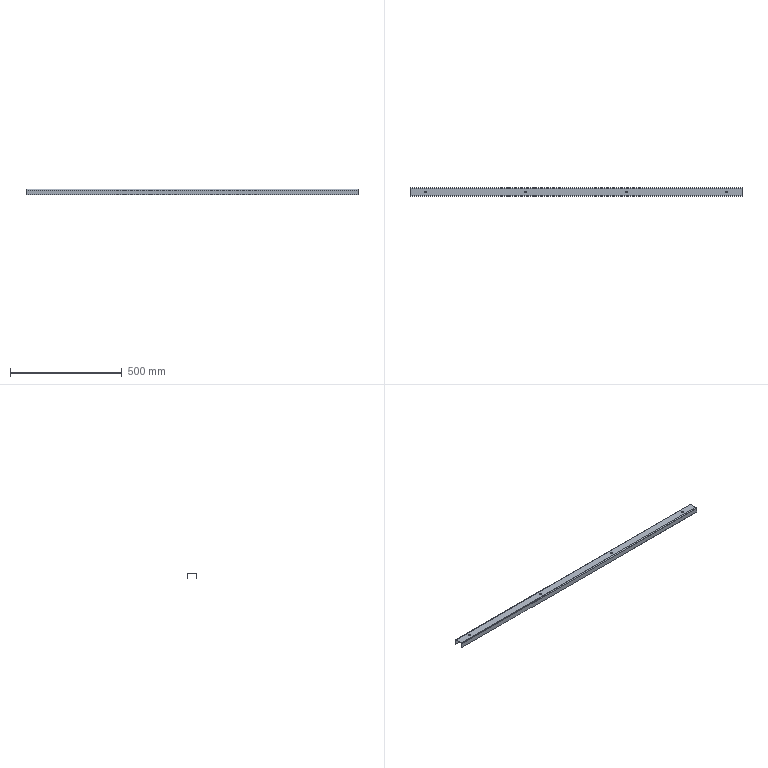Part | STEP file | SYL_0392D6J1SYL0380DJ10-1081048 | 1 solid | 30 faces | box 1488 x 40 x 25 mm | volume 247870 mm3 | plane 18 | cylinder 12 | commonest cylinder face diameters 8 x10 4 x2
STEP:
#1=CARTESIAN_POINT('',(-679.,0.,10.5));
#2=VERTEX_POINT('',#1);
#3=CARTESIAN_POINT('',(-679.,0.,12.5));
#4=VERTEX_POINT('',#3);
#5=CARTESIAN_POINT('',(-679.,0.,12.5));
#6=DIRECTION('',(0.,0.,1.));
#7=VECTOR('',#6,1000.);
#8=LINE('',#5,#7);
#9=EDGE_CURVE('',#2,#4,#8,.T.);
#10=ORIENTED_EDGE('',*,*,#9,.F.);
#11=CARTESIAN_POINT('',(-671.,0.,10.5));
#12=VERTEX_POINT('',#11);
#13=CARTESIAN_POINT('',(-675.,0.,10.5));
#14=DIRECTION('',(0.,0.,-1.));
#15=DIRECTION('',(-1.,0.,0.));
#16=AXIS2_PLACEMENT_3D('',#13,#14,#15);
#17=CIRCLE('',#16,4.);
#18=EDGE_CURVE('',#2,#12,#17,.T.);
#19=ORIENTED_EDGE('',*,*,#18,.T.);
#20=CARTESIAN_POINT('',(-671.,0.,12.5));
#21=VERTEX_POINT('',#20);
#22=CARTESIAN_POINT('',(-671.,0.,12.5));
#23=DIRECTION('',(0.,0.,1.));
#24=VECTOR('',#23,1000.);
#25=LINE('',#22,#24);
#26=EDGE_CURVE('',#12,#21,#25,.T.);
#27=ORIENTED_EDGE('',*,*,#26,.T.);
#28=CARTESIAN_POINT('',(-675.,0.,12.5));
#29=DIRECTION('',(0.,0.,-1.));
#30=DIRECTION('',(-1.,0.,0.));
#31=AXIS2_PLACEMENT_3D('',#28,#29,#30);
#32=CIRCLE('',#31,4.);
#33=EDGE_CURVE('',#4,#21,#32,.T.);
#34=ORIENTED_EDGE('',*,*,#33,.F.);
#35=EDGE_LOOP('',(#10,#19,#27,#34));
#36=FACE_OUTER_BOUND('',#35,.T.);
#37=CARTESIAN_POINT('',(-675.,0.,12.5));
#38=DIRECTION('',(0.,0.,1.));
#39=DIRECTION('',(1.,0.,0.));
#40=AXIS2_PLACEMENT_3D('',#37,#38,#39);
#41=CYLINDRICAL_SURFACE('',#40,4.);
#42=ADVANCED_FACE('',(#36),#41,.F.);
#43=CARTESIAN_POINT('',(-229.,0.,10.5));
#44=VERTEX_POINT('',#43);
#45=CARTESIAN_POINT('',(-229.,0.,12.5));
#46=VERTEX_POINT('',#45);
#47=CARTESIAN_POINT('',(-229.,0.,12.5));
#48=DIRECTION('',(0.,0.,1.));
#49=VECTOR('',#48,1000.);
#50=LINE('',#47,#49);
#51=EDGE_CURVE('',#44,#46,#50,.T.);
#52=ORIENTED_EDGE('',*,*,#51,.F.);
#53=CARTESIAN_POINT('',(-221.,0.,10.5));
#54=VERTEX_POINT('',#53);
#55=CARTESIAN_POINT('',(-225.,0.,10.5));
#56=DIRECTION('',(0.,0.,-1.));
#57=DIRECTION('',(-1.,0.,0.));
#58=AXIS2_PLACEMENT_3D('',#55,#56,#57);
#59=CIRCLE('',#58,4.);
#60=EDGE_CURVE('',#44,#54,#59,.T.);
#61=ORIENTED_EDGE('',*,*,#60,.T.);
#62=CARTESIAN_POINT('',(-221.,0.,12.5));
#63=VERTEX_POINT('',#62);
#64=CARTESIAN_POINT('',(-221.,0.,12.5));
#65=DIRECTION('',(0.,0.,1.));
#66=VECTOR('',#65,1000.);
#67=LINE('',#64,#66);
#68=EDGE_CURVE('',#54,#63,#67,.T.);
#69=ORIENTED_EDGE('',*,*,#68,.T.);
#70=CARTESIAN_POINT('',(-225.,0.,12.5));
#71=DIRECTION('',(0.,0.,-1.));
#72=DIRECTION('',(-1.,0.,0.));
#73=AXIS2_PLACEMENT_3D('',#70,#71,#72);
#74=CIRCLE('',#73,4.);
#75=EDGE_CURVE('',#46,#63,#74,.T.);
#76=ORIENTED_EDGE('',*,*,#75,.F.);
#77=EDGE_LOOP('',(#52,#61,#69,#76));
#78=FACE_OUTER_BOUND('',#77,.T.);
#79=CARTESIAN_POINT('',(-225.,0.,12.5));
#80=DIRECTION('',(0.,0.,1.));
#81=DIRECTION('',(1.,0.,0.));
#82=AXIS2_PLACEMENT_3D('',#79,#80,#81);
#83=CYLINDRICAL_SURFACE('',#82,4.);
#84=ADVANCED_FACE('',(#78),#83,.F.);
#85=CARTESIAN_POINT('',(221.,0.,10.5));
#86=VERTEX_POINT('',#85);
#87=CARTESIAN_POINT('',(221.,0.,12.5));
#88=VERTEX_POINT('',#87);
#89=CARTESIAN_POINT('',(221.,0.,12.5));
#90=DIRECTION('',(0.,0.,1.));
#91=VECTOR('',#90,1000.);
#92=LINE('',#89,#91);
#93=EDGE_CURVE('',#86,#88,#92,.T.);
#94=ORIENTED_EDGE('',*,*,#93,.F.);
#95=CARTESIAN_POINT('',(229.,0.,10.5));
#96=VERTEX_POINT('',#95);
#97=CARTESIAN_POINT('',(225.,0.,10.5));
#98=DIRECTION('',(0.,0.,-1.));
#99=DIRECTION('',(-1.,0.,0.));
#100=AXIS2_PLACEMENT_3D('',#97,#98,#99);
#101=CIRCLE('',#100,4.);
#102=EDGE_CURVE('',#86,#96,#101,.T.);
#103=ORIENTED_EDGE('',*,*,#102,.T.);
#104=CARTESIAN_POINT('',(229.,0.,12.5));
#105=VERTEX_POINT('',#104);
#106=CARTESIAN_POINT('',(229.,0.,12.5));
#107=DIRECTION('',(0.,0.,1.));
#108=VECTOR('',#107,1000.);
#109=LINE('',#106,#108);
#110=EDGE_CURVE('',#96,#105,#109,.T.);
#111=ORIENTED_EDGE('',*,*,#110,.T.);
#112=CARTESIAN_POINT('',(225.,0.,12.5));
#113=DIRECTION('',(0.,0.,-1.));
#114=DIRECTION('',(-1.,0.,0.));
#115=AXIS2_PLACEMENT_3D('',#112,#113,#114);
#116=CIRCLE('',#115,4.);
#117=EDGE_CURVE('',#88,#105,#116,.T.);
#118=ORIENTED_EDGE('',*,*,#117,.F.);
#119=EDGE_LOOP('',(#94,#103,#111,#118));
#120=FACE_OUTER_BOUND('',#119,.T.);
#121=CARTESIAN_POINT('',(225.,0.,12.5));
#122=DIRECTION('',(0.,0.,1.));
#123=DIRECTION('',(1.,0.,0.));
#124=AXIS2_PLACEMENT_3D('',#121,#122,#123);
#125=CYLINDRICAL_SURFACE('',#124,4.);
#126=ADVANCED_FACE('',(#120),#125,.F.);
#127=CARTESIAN_POINT('',(671.,0.,10.5));
#128=VERTEX_POINT('',#127);
#129=CARTESIAN_POINT('',(671.,0.,12.5));
#130=VERTEX_POINT('',#129);
#131=CARTESIAN_POINT('',(671.,0.,12.5));
#132=DIRECTION('',(0.,0.,1.));
#133=VECTOR('',#132,1000.);
#134=LINE('',#131,#133);
#135=EDGE_CURVE('',#128,#130,#134,.T.);
#136=ORIENTED_EDGE('',*,*,#135,.F.);
#137=CARTESIAN_POINT('',(679.,0.,10.5));
#138=VERTEX_POINT('',#137);
#139=CARTESIAN_POINT('',(675.,0.,10.5));
#140=DIRECTION('',(0.,0.,-1.));
#141=DIRECTION('',(-1.,0.,0.));
#142=AXIS2_PLACEMENT_3D('',#139,#140,#141);
#143=CIRCLE('',#142,4.);
#144=EDGE_CURVE('',#128,#138,#143,.T.);
#145=ORIENTED_EDGE('',*,*,#144,.T.);
#146=CARTESIAN_POINT('',(679.,0.,12.5));
#147=VERTEX_POINT('',#146);
#148=CARTESIAN_POINT('',(679.,0.,12.5));
#149=DIRECTION('',(0.,0.,1.));
#150=VECTOR('',#149,1000.);
#151=LINE('',#148,#150);
#152=EDGE_CURVE('',#138,#147,#151,.T.);
#153=ORIENTED_EDGE('',*,*,#152,.T.);
#154=CARTESIAN_POINT('',(675.,0.,12.5));
#155=DIRECTION('',(0.,0.,-1.));
#156=DIRECTION('',(-1.,0.,0.));
#157=AXIS2_PLACEMENT_3D('',#154,#155,#156);
#158=CIRCLE('',#157,4.);
#159=EDGE_CURVE('',#130,#147,#158,.T.);
#160=ORIENTED_EDGE('',*,*,#159,.F.);
#161=EDGE_LOOP('',(#136,#145,#153,#160));
#162=FACE_OUTER_BOUND('',#161,.T.);
#163=CARTESIAN_POINT('',(675.,0.,12.5));
#164=DIRECTION('',(0.,0.,1.));
#165=DIRECTION('',(1.,0.,0.));
#166=AXIS2_PLACEMENT_3D('',#163,#164,#165);
#167=CYLINDRICAL_SURFACE('',#166,4.);
#168=ADVANCED_FACE('',(#162),#167,.F.);
#169=CARTESIAN_POINT('',(744.,18.,-12.5));
#170=VERTEX_POINT('',#169);
#171=CARTESIAN_POINT('',(744.,20.,-12.5));
#172=VERTEX_POINT('',#171);
#173=CARTESIAN_POINT('',(744.,20.,-12.5));
#174=DIRECTION('',(0.,1.,0.));
#175=VECTOR('',#174,1000.);
#176=LINE('',#173,#175);
#177=EDGE_CURVE('',#170,#172,#176,.T.);
#178=ORIENTED_EDGE('',*,*,#177,.F.);
#179=CARTESIAN_POINT('',(-744.,18.,-12.5));
#180=VERTEX_POINT('',#179);
#181=CARTESIAN_POINT('',(-744.,18.,-12.5));
#182=DIRECTION('',(1.,0.,0.));
#183=VECTOR('',#182,1000.);
#184=LINE('',#181,#183);
#185=EDGE_CURVE('',#180,#170,#184,.T.);
#186=ORIENTED_EDGE('',*,*,#185,.F.);
#187=CARTESIAN_POINT('',(-744.,20.,-12.5));
#188=VERTEX_POINT('',#187);
#189=CARTESIAN_POINT('',(-744.,20.,-12.5));
#190=DIRECTION('',(0.,1.,0.));
#191=VECTOR('',#190,1000.);
#192=LINE('',#189,#191);
#193=EDGE_CURVE('',#180,#188,#192,.T.);
#194=ORIENTED_EDGE('',*,*,#193,.T.);
#195=CARTESIAN_POINT('',(-744.,20.,-12.5));
#196=DIRECTION('',(1.,0.,0.));
#197=VECTOR('',#196,1000.);
#198=LINE('',#195,#197);
#199=EDGE_CURVE('',#188,#172,#198,.T.);
#200=ORIENTED_EDGE('',*,*,#199,.T.);
#201=EDGE_LOOP('',(#178,#186,#194,#200));
#202=FACE_OUTER_BOUND('',#201,.T.);
#203=CARTESIAN_POINT('',(-744.,20.,-12.5));
#204=DIRECTION('',(0.,0.,1.));
#205=DIRECTION('',(1.,0.,0.));
#206=AXIS2_PLACEMENT_3D('',#203,#204,#205);
#207=PLANE('',#206);
#208=ADVANCED_FACE('',(#202),#207,.F.);
#209=ORIENTED_EDGE('',*,*,#193,.F.);
#210=CARTESIAN_POINT('',(-744.,18.,8.5));
#211=VERTEX_POINT('',#210);
#212=CARTESIAN_POINT('',(-744.,18.,-12.5));
#213=DIRECTION('',(0.,0.,-1.));
#214=VECTOR('',#213,1000.);
#215=LINE('',#212,#214);
#216=EDGE_CURVE('',#211,#180,#215,.T.);
#217=ORIENTED_EDGE('',*,*,#216,.F.);
#218=CARTESIAN_POINT('',(-744.,20.,8.5));
#219=VERTEX_POINT('',#218);
#220=CARTESIAN_POINT('',(-744.,20.,8.5));
#221=DIRECTION('',(0.,1.,0.));
#222=VECTOR('',#221,1000.);
#223=LINE('',#220,#222);
#224=EDGE_CURVE('',#211,#219,#223,.T.);
#225=ORIENTED_EDGE('',*,*,#224,.T.);
#226=CARTESIAN_POINT('',(-744.,20.,8.5));
#227=DIRECTION('',(0.,0.,-1.));
#228=VECTOR('',#227,1000.);
#229=LINE('',#226,#228);
#230=EDGE_CURVE('',#219,#188,#229,.T.);
#231=ORIENTED_EDGE('',*,*,#230,.T.);
#232=EDGE_LOOP('',(#209,#217,#225,#231));
#233=FACE_OUTER_BOUND('',#232,.T.);
#234=CARTESIAN_POINT('',(-744.,20.,8.5));
#235=DIRECTION('',(1.,0.,0.));
#236=DIRECTION('',(0.,0.,-1.));
#237=AXIS2_PLACEMENT_3D('',#234,#235,#236);
#238=PLANE('',#237);
#239=ADVANCED_FACE('',(#233),#238,.F.);
#240=ORIENTED_EDGE('',*,*,#224,.F.);
#241=CARTESIAN_POINT('',(-744.,16.,10.5));
#242=VERTEX_POINT('',#241);
#243=CARTESIAN_POINT('',(-744.,16.,8.5));
#244=DIRECTION('',(-1.,0.,0.));
#245=DIRECTION('',(0.,0.,1.));
#246=AXIS2_PLACEMENT_3D('',#243,#244,#245);
#247=CIRCLE('',#246,2.);
#248=EDGE_CURVE('',#242,#211,#247,.T.);
#249=ORIENTED_EDGE('',*,*,#248,.F.);
#250=CARTESIAN_POINT('',(-744.,16.,12.5));
#251=VERTEX_POINT('',#250);
#252=CARTESIAN_POINT('',(-744.,16.,12.5));
#253=DIRECTION('',(0.,0.,1.));
#254=VECTOR('',#253,1000.);
#255=LINE('',#252,#254);
#256=EDGE_CURVE('',#242,#251,#255,.T.);
#257=ORIENTED_EDGE('',*,*,#256,.T.);
#258=CARTESIAN_POINT('',(-744.,16.,8.5));
#259=DIRECTION('',(-1.,0.,0.));
#260=DIRECTION('',(0.,0.,1.));
#261=AXIS2_PLACEMENT_3D('',#258,#259,#260);
#262=CIRCLE('',#261,4.);
#263=EDGE_CURVE('',#251,#219,#262,.T.);
#264=ORIENTED_EDGE('',*,*,#263,.T.);
#265=EDGE_LOOP('',(#240,#249,#257,#264));
#266=FACE_OUTER_BOUND('',#265,.T.);
#267=CARTESIAN_POINT('',(-744.,16.,8.5));
#268=DIRECTION('',(1.,0.,0.));
#269=DIRECTION('',(0.,0.,-1.));
#270=AXIS2_PLACEMENT_3D('',#267,#268,#269);
#271=PLANE('',#270);
#272=ADVANCED_FACE('',(#266),#271,.F.);
#273=ORIENTED_EDGE('',*,*,#256,.F.);
#274=CARTESIAN_POINT('',(-744.,-16.,10.5));
#275=VERTEX_POINT('',#274);
#276=CARTESIAN_POINT('',(-744.,20.,10.5));
#277=DIRECTION('',(0.,1.,0.));
#278=VECTOR('',#277,1000.);
#279=LINE('',#276,#278);
#280=EDGE_CURVE('',#275,#242,#279,.T.);
#281=ORIENTED_EDGE('',*,*,#280,.F.);
#282=CARTESIAN_POINT('',(-744.,-16.,12.5));
#283=VERTEX_POINT('',#282);
#284=CARTESIAN_POINT('',(-744.,-16.,12.5));
#285=DIRECTION('',(0.,0.,1.));
#286=VECTOR('',#285,1000.);
#287=LINE('',#284,#286);
#288=EDGE_CURVE('',#275,#283,#287,.T.);
#289=ORIENTED_EDGE('',*,*,#288,.T.);
#290=CARTESIAN_POINT('',(-744.,-16.,12.5));
#291=DIRECTION('',(0.,1.,0.));
#292=VECTOR('',#291,1000.);
#293=LINE('',#290,#292);
#294=EDGE_CURVE('',#283,#251,#293,.T.);
#295=ORIENTED_EDGE('',*,*,#294,.T.);
#296=EDGE_LOOP('',(#273,#281,#289,#295));
#297=FACE_OUTER_BOUND('',#296,.T.);
#298=CARTESIAN_POINT('',(-744.,-16.,12.5));
#299=DIRECTION('',(1.,0.,0.));
#300=DIRECTION('',(0.,1.,0.));
#301=AXIS2_PLACEMENT_3D('',#298,#299,#300);
#302=PLANE('',#301);
#303=ADVANCED_FACE('',(#297),#302,.F.);
#304=ORIENTED_EDGE('',*,*,#288,.F.);
#305=CARTESIAN_POINT('',(-744.,-18.,8.5));
#306=VERTEX_POINT('',#305);
#307=CARTESIAN_POINT('',(-744.,-16.,8.5));
#308=DIRECTION('',(-1.,0.,0.));
#309=DIRECTION('',(0.,0.,1.));
#310=AXIS2_PLACEMENT_3D('',#307,#308,#309);
#311=CIRCLE('',#310,2.);
#312=EDGE_CURVE('',#306,#275,#311,.T.);
#313=ORIENTED_EDGE('',*,*,#312,.F.);
#314=CARTESIAN_POINT('',(-744.,-20.,8.5));
#315=VERTEX_POINT('',#314);
#316=CARTESIAN_POINT('',(-744.,-20.,8.5));
#317=DIRECTION('',(0.,-1.,0.));
#318=VECTOR('',#317,1000.);
#319=LINE('',#316,#318);
#320=EDGE_CURVE('',#306,#315,#319,.T.);
#321=ORIENTED_EDGE('',*,*,#320,.T.);
#322=CARTESIAN_POINT('',(-744.,-16.,8.5));
#323=DIRECTION('',(-1.,0.,0.));
#324=DIRECTION('',(0.,-1.,0.));
#325=AXIS2_PLACEMENT_3D('',#322,#323,#324);
#326=CIRCLE('',#325,4.);
#327=EDGE_CURVE('',#315,#283,#326,.T.);
#328=ORIENTED_EDGE('',*,*,#327,.T.);
#329=EDGE_LOOP('',(#304,#313,#321,#328));
#330=FACE_OUTER_BOUND('',#329,.T.);
#331=CARTESIAN_POINT('',(-744.,-16.,8.5));
#332=DIRECTION('',(1.,0.,0.));
#333=DIRECTION('',(0.,0.,-1.));
#334=AXIS2_PLACEMENT_3D('',#331,#332,#333);
#335=PLANE('',#334);
#336=ADVANCED_FACE('',(#330),#335,.F.);
#337=ORIENTED_EDGE('',*,*,#320,.F.);
#338=CARTESIAN_POINT('',(-744.,-18.,-12.5));
#339=VERTEX_POINT('',#338);
#340=CARTESIAN_POINT('',(-744.,-18.,12.5));
#341=DIRECTION('',(0.,0.,1.));
#342=VECTOR('',#341,1000.);
#343=LINE('',#340,#342);
#344=EDGE_CURVE('',#339,#306,#343,.T.);
#345=ORIENTED_EDGE('',*,*,#344,.F.);
#346=CARTESIAN_POINT('',(-744.,-20.,-12.5));
#347=VERTEX_POINT('',#346);
#348=CARTESIAN_POINT('',(-744.,-20.,-12.5));
#349=DIRECTION('',(0.,-1.,0.));
#350=VECTOR('',#349,1000.);
#351=LINE('',#348,#350);
#352=EDGE_CURVE('',#339,#347,#351,.T.);
#353=ORIENTED_EDGE('',*,*,#352,.T.);
#354=CARTESIAN_POINT('',(-744.,-20.,-12.5));
#355=DIRECTION('',(0.,0.,1.));
#356=VECTOR('',#355,1000.);
#357=LINE('',#354,#356);
#358=EDGE_CURVE('',#347,#315,#357,.T.);
#359=ORIENTED_EDGE('',*,*,#358,.T.);
#360=EDGE_LOOP('',(#337,#345,#353,#359));
#361=FACE_OUTER_BOUND('',#360,.T.);
#362=CARTESIAN_POINT('',(-744.,-20.,-12.5));
#363=DIRECTION('',(1.,0.,0.));
#364=DIRECTION('',(0.,0.,1.));
#365=AXIS2_PLACEMENT_3D('',#362,#363,#364);
#366=PLANE('',#365);
#367=ADVANCED_FACE('',(#361),#366,.F.);
#368=ORIENTED_EDGE('',*,*,#352,.F.);
#369=CARTESIAN_POINT('',(744.,-18.,-12.5));
#370=VERTEX_POINT('',#369);
#371=CARTESIAN_POINT('',(-744.,-18.,-12.5));
#372=DIRECTION('',(-1.,0.,0.));
#373=VECTOR('',#372,1000.);
#374=LINE('',#371,#373);
#375=EDGE_CURVE('',#370,#339,#374,.T.);
#376=ORIENTED_EDGE('',*,*,#375,.F.);
#377=CARTESIAN_POINT('',(744.,-20.,-12.5));
#378=VERTEX_POINT('',#377);
#379=CARTESIAN_POINT('',(744.,-20.,-12.5));
#380=DIRECTION('',(0.,-1.,0.));
#381=VECTOR('',#380,1000.);
#382=LINE('',#379,#381);
#383=EDGE_CURVE('',#370,#378,#382,.T.);
#384=ORIENTED_EDGE('',*,*,#383,.T.);
#385=CARTESIAN_POINT('',(744.,-20.,-12.5));
#386=DIRECTION('',(-1.,0.,0.));
#387=VECTOR('',#386,1000.);
#388=LINE('',#385,#387);
#389=EDGE_CURVE('',#378,#347,#388,.T.);
#390=ORIENTED_EDGE('',*,*,#389,.T.);
#391=EDGE_LOOP('',(#368,#376,#384,#390));
#392=FACE_OUTER_BOUND('',#391,.T.);
#393=CARTESIAN_POINT('',(744.,-20.,-12.5));
#394=DIRECTION('',(0.,0.,1.));
#395=DIRECTION('',(-1.,0.,0.));
#396=AXIS2_PLACEMENT_3D('',#393,#394,#395);
#397=PLANE('',#396);
#398=ADVANCED_FACE('',(#392),#397,.F.);
#399=ORIENTED_EDGE('',*,*,#383,.F.);
#400=CARTESIAN_POINT('',(744.,-18.,8.5));
#401=VERTEX_POINT('',#400);
#402=CARTESIAN_POINT('',(744.,-18.,12.5));
#403=DIRECTION('',(0.,0.,-1.));
#404=VECTOR('',#403,1000.);
#405=LINE('',#402,#404);
#406=EDGE_CURVE('',#401,#370,#405,.T.);
#407=ORIENTED_EDGE('',*,*,#406,.F.);
#408=CARTESIAN_POINT('',(744.,-20.,8.5));
#409=VERTEX_POINT('',#408);
#410=CARTESIAN_POINT('',(744.,-20.,8.5));
#411=DIRECTION('',(0.,-1.,0.));
#412=VECTOR('',#411,1000.);
#413=LINE('',#410,#412);
#414=EDGE_CURVE('',#401,#409,#413,.T.);
#415=ORIENTED_EDGE('',*,*,#414,.T.);
#416=CARTESIAN_POINT('',(744.,-20.,8.5));
#417=DIRECTION('',(0.,0.,-1.));
#418=VECTOR('',#417,1000.);
#419=LINE('',#416,#418);
#420=EDGE_CURVE('',#409,#378,#419,.T.);
#421=ORIENTED_EDGE('',*,*,#420,.T.);
#422=EDGE_LOOP('',(#399,#407,#415,#421));
#423=FACE_OUTER_BOUND('',#422,.T.);
#424=CARTESIAN_POINT('',(744.,-20.,8.5));
#425=DIRECTION('',(-1.,0.,0.));
#426=DIRECTION('',(0.,0.,-1.));
#427=AXIS2_PLACEMENT_3D('',#424,#425,#426);
#428=PLANE('',#427);
#429=ADVANCED_FACE('',(#423),#428,.F.);
#430=ORIENTED_EDGE('',*,*,#414,.F.);
#431=CARTESIAN_POINT('',(744.,-16.,10.5));
#432=VERTEX_POINT('',#431);
#433=CARTESIAN_POINT('',(744.,-16.,8.5));
#434=DIRECTION('',(1.,0.,0.));
#435=DIRECTION('',(0.,0.,1.));
#436=AXIS2_PLACEMENT_3D('',#433,#434,#435);
#437=CIRCLE('',#436,2.);
#438=EDGE_CURVE('',#432,#401,#437,.T.);
#439=ORIENTED_EDGE('',*,*,#438,.F.);
#440=CARTESIAN_POINT('',(744.,-16.,12.5));
#441=VERTEX_POINT('',#440);
#442=CARTESIAN_POINT('',(744.,-16.,12.5));
#443=DIRECTION('',(0.,0.,1.));
#444=VECTOR('',#443,1000.);
#445=LINE('',#442,#444);
#446=EDGE_CURVE('',#432,#441,#445,.T.);
#447=ORIENTED_EDGE('',*,*,#446,.T.);
#448=CARTESIAN_POINT('',(744.,-16.,8.5));
#449=DIRECTION('',(1.,0.,0.));
#450=DIRECTION('',(0.,0.,1.));
#451=AXIS2_PLACEMENT_3D('',#448,#449,#450);
#452=CIRCLE('',#451,4.);
#453=EDGE_CURVE('',#441,#409,#452,.T.);
#454=ORIENTED_EDGE('',*,*,#453,.T.);
#455=EDGE_LOOP('',(#430,#439,#447,#454));
#456=FACE_OUTER_BOUND('',#455,.T.);
#457=CARTESIAN_POINT('',(744.,-16.,8.5));
#458=DIRECTION('',(-1.,0.,0.));
#459=DIRECTION('',(0.,0.,1.));
#460=AXIS2_PLACEMENT_3D('',#457,#458,#459);
#461=PLANE('',#460);
#462=ADVANCED_FACE('',(#456),#461,.F.);
#463=ORIENTED_EDGE('',*,*,#446,.F.);
#464=CARTESIAN_POINT('',(744.,16.,10.5));
#465=VERTEX_POINT('',#464);
#466=CARTESIAN_POINT('',(744.,20.,10.5));
#467=DIRECTION('',(0.,-1.,0.));
#468=VECTOR('',#467,1000.);
#469=LINE('',#466,#468);
#470=EDGE_CURVE('',#465,#432,#469,.T.);
#471=ORIENTED_EDGE('',*,*,#470,.F.);
#472=CARTESIAN_POINT('',(744.,16.,12.5));
#473=VERTEX_POINT('',#472);
#474=CARTESIAN_POINT('',(744.,16.,12.5));
#475=DIRECTION('',(0.,0.,1.));
#476=VECTOR('',#475,1000.);
#477=LINE('',#474,#476);
#478=EDGE_CURVE('',#465,#473,#477,.T.);
#479=ORIENTED_EDGE('',*,*,#478,.T.);
#480=CARTESIAN_POINT('',(744.,16.,12.5));
#481=DIRECTION('',(0.,-1.,0.));
#482=VECTOR('',#481,1000.);
#483=LINE('',#480,#482);
#484=EDGE_CURVE('',#473,#441,#483,.T.);
#485=ORIENTED_EDGE('',*,*,#484,.T.);
#486=EDGE_LOOP('',(#463,#471,#479,#485));
#487=FACE_OUTER_BOUND('',#486,.T.);
#488=CARTESIAN_POINT('',(744.,16.,12.5));
#489=DIRECTION('',(-1.,0.,0.));
#490=DIRECTION('',(0.,-1.,0.));
#491=AXIS2_PLACEMENT_3D('',#488,#489,#490);
#492=PLANE('',#491);
#493=ADVANCED_FACE('',(#487),#492,.F.);
#494=ORIENTED_EDGE('',*,*,#478,.F.);
#495=CARTESIAN_POINT('',(744.,18.,8.5));
#496=VERTEX_POINT('',#495);
#497=CARTESIAN_POINT('',(744.,16.,8.5));
#498=DIRECTION('',(1.,0.,0.));
#499=DIRECTION('',(0.,0.,1.));
#500=AXIS2_PLACEMENT_3D('',#497,#498,#499);
#501=CIRCLE('',#500,2.);
#502=EDGE_CURVE('',#496,#465,#501,.T.);
#503=ORIENTED_EDGE('',*,*,#502,.F.);
#504=CARTESIAN_POINT('',(744.,20.,8.5));
#505=VERTEX_POINT('',#504);
#506=CARTESIAN_POINT('',(744.,20.,8.5));
#507=DIRECTION('',(0.,1.,0.));
#508=VECTOR('',#507,1000.);
#509=LINE('',#506,#508);
#510=EDGE_CURVE('',#496,#505,#509,.T.);
#511=ORIENTED_EDGE('',*,*,#510,.T.);
#512=CARTESIAN_POINT('',(744.,16.,8.5));
#513=DIRECTION('',(1.,0.,0.));
#514=DIRECTION('',(0.,1.,0.));
#515=AXIS2_PLACEMENT_3D('',#512,#513,#514);
#516=CIRCLE('',#515,4.);
#517=EDGE_CURVE('',#505,#473,#516,.T.);
#518=ORIENTED_EDGE('',*,*,#517,.T.);
#519=EDGE_LOOP('',(#494,#503,#511,#518));
#520=FACE_OUTER_BOUND('',#519,.T.);
#521=CARTESIAN_POINT('',(744.,16.,8.5));
#522=DIRECTION('',(-1.,0.,0.));
#523=DIRECTION('',(0.,0.,1.));
#524=AXIS2_PLACEMENT_3D('',#521,#522,#523);
#525=PLANE('',#524);
#526=ADVANCED_FACE('',(#520),#525,.F.);
#527=CARTESIAN_POINT('',(675.,0.,10.5));
#528=DIRECTION('',(0.,0.,-1.));
#529=DIRECTION('',(-1.,0.,0.));
#530=AXIS2_PLACEMENT_3D('',#527,#528,#529);
#531=CIRCLE('',#530,4.);
#532=EDGE_CURVE('',#138,#128,#531,.T.);
#533=ORIENTED_EDGE('',*,*,#532,.T.);
#534=ORIENTED_EDGE('',*,*,#135,.T.);
#535=CARTESIAN_POINT('',(675.,0.,12.5));
#536=DIRECTION('',(0.,0.,-1.));
#537=DIRECTION('',(1.,0.,0.));
#538=AXIS2_PLACEMENT_3D('',#535,#536,#537);
#539=CIRCLE('',#538,4.);
#540=EDGE_CURVE('',#147,#130,#539,.T.);
#541=ORIENTED_EDGE('',*,*,#540,.F.);
#542=ORIENTED_EDGE('',*,*,#152,.F.);
#543=EDGE_LOOP('',(#533,#534,#541,#542));
#544=FACE_OUTER_BOUND('',#543,.T.);
#545=CARTESIAN_POINT('',(675.,0.,12.5));
#546=DIRECTION('',(0.,0.,1.));
#547=DIRECTION('',(1.,0.,0.));
#548=AXIS2_PLACEMENT_3D('',#545,#546,#547);
#549=CYLINDRICAL_SURFACE('',#548,4.);
#550=ADVANCED_FACE('',(#544),#549,.F.);
#551=CARTESIAN_POINT('',(225.,0.,10.5));
#552=DIRECTION('',(0.,0.,-1.));
#553=DIRECTION('',(-1.,0.,0.));
#554=AXIS2_PLACEMENT_3D('',#551,#552,#553);
#555=CIRCLE('',#554,4.);
#556=EDGE_CURVE('',#96,#86,#555,.T.);
#557=ORIENTED_EDGE('',*,*,#556,.T.);
#558=ORIENTED_EDGE('',*,*,#93,.T.);
#559=CARTESIAN_POINT('',(225.,0.,12.5));
#560=DIRECTION('',(0.,0.,-1.));
#561=DIRECTION('',(1.,0.,0.));
#562=AXIS2_PLACEMENT_3D('',#559,#560,#561);
#563=CIRCLE('',#562,4.);
#564=EDGE_CURVE('',#105,#88,#563,.T.);
#565=ORIENTED_EDGE('',*,*,#564,.F.);
#566=ORIENTED_EDGE('',*,*,#110,.F.);
#567=EDGE_LOOP('',(#557,#558,#565,#566));
#568=FACE_OUTER_BOUND('',#567,.T.);
#569=CARTESIAN_POINT('',(225.,0.,12.5));
#570=DIRECTION('',(0.,0.,1.));
#571=DIRECTION('',(1.,0.,0.));
#572=AXIS2_PLACEMENT_3D('',#569,#570,#571);
#573=CYLINDRICAL_SURFACE('',#572,4.);
#574=ADVANCED_FACE('',(#568),#573,.F.);
#575=CARTESIAN_POINT('',(-225.,0.,10.5));
#576=DIRECTION('',(0.,0.,-1.));
#577=DIRECTION('',(-1.,0.,0.));
#578=AXIS2_PLACEMENT_3D('',#575,#576,#577);
#579=CIRCLE('',#578,4.);
#580=EDGE_CURVE('',#54,#44,#579,.T.);
#581=ORIENTED_EDGE('',*,*,#580,.T.);
#582=ORIENTED_EDGE('',*,*,#51,.T.);
#583=CARTESIAN_POINT('',(-225.,0.,12.5));
#584=DIRECTION('',(0.,0.,-1.));
#585=DIRECTION('',(1.,0.,0.));
#586=AXIS2_PLACEMENT_3D('',#583,#584,#585);
#587=CIRCLE('',#586,4.);
#588=EDGE_CURVE('',#63,#46,#587,.T.);
#589=ORIENTED_EDGE('',*,*,#588,.F.);
#590=ORIENTED_EDGE('',*,*,#68,.F.);
#591=EDGE_LOOP('',(#581,#582,#589,#590));
#592=FACE_OUTER_BOUND('',#591,.T.);
#593=CARTESIAN_POINT('',(-225.,0.,12.5));
#594=DIRECTION('',(0.,0.,1.));
#595=DIRECTION('',(1.,0.,0.));
#596=AXIS2_PLACEMENT_3D('',#593,#594,#595);
#597=CYLINDRICAL_SURFACE('',#596,4.);
#598=ADVANCED_FACE('',(#592),#597,.F.);
#599=CARTESIAN_POINT('',(-675.,0.,10.5));
#600=DIRECTION('',(0.,0.,-1.));
#601=DIRECTION('',(-1.,0.,0.));
#602=AXIS2_PLACEMENT_3D('',#599,#600,#601);
#603=CIRCLE('',#602,4.);
#604=EDGE_CURVE('',#12,#2,#603,.T.);
#605=ORIENTED_EDGE('',*,*,#604,.T.);
#606=ORIENTED_EDGE('',*,*,#9,.T.);
#607=CARTESIAN_POINT('',(-675.,0.,12.5));
#608=DIRECTION('',(0.,0.,-1.));
#609=DIRECTION('',(1.,0.,0.));
#610=AXIS2_PLACEMENT_3D('',#607,#608,#609);
#611=CIRCLE('',#610,4.);
#612=EDGE_CURVE('',#21,#4,#611,.T.);
#613=ORIENTED_EDGE('',*,*,#612,.F.);
#614=ORIENTED_EDGE('',*,*,#26,.F.);
#615=EDGE_LOOP('',(#605,#606,#613,#614));
#616=FACE_OUTER_BOUND('',#615,.T.);
#617=CARTESIAN_POINT('',(-675.,0.,12.5));
#618=DIRECTION('',(0.,0.,1.));
#619=DIRECTION('',(1.,0.,0.));
#620=AXIS2_PLACEMENT_3D('',#617,#618,#619);
#621=CYLINDRICAL_SURFACE('',#620,4.);
#622=ADVANCED_FACE('',(#616),#621,.F.);
#623=CARTESIAN_POINT('',(744.,18.,-12.5));
#624=DIRECTION('',(0.,0.,1.));
#625=VECTOR('',#624,1000.);
#626=LINE('',#623,#625);
#627=EDGE_CURVE('',#170,#496,#626,.T.);
#628=ORIENTED_EDGE('',*,*,#627,.F.);
#629=ORIENTED_EDGE('',*,*,#177,.T.);
#630=CARTESIAN_POINT('',(744.,20.,-12.5));
#631=DIRECTION('',(0.,0.,1.));
#632=VECTOR('',#631,1000.);
#633=LINE('',#630,#632);
#634=EDGE_CURVE('',#172,#505,#633,.T.);
#635=ORIENTED_EDGE('',*,*,#634,.T.);
#636=ORIENTED_EDGE('',*,*,#510,.F.);
#637=EDGE_LOOP('',(#628,#629,#635,#636));
#638=FACE_OUTER_BOUND('',#637,.T.);
#639=CARTESIAN_POINT('',(744.,20.,-12.5));
#640=DIRECTION('',(-1.,0.,0.));
#641=DIRECTION('',(0.,0.,1.));
#642=AXIS2_PLACEMENT_3D('',#639,#640,#641);
#643=PLANE('',#642);
#644=ADVANCED_FACE('',(#638),#643,.F.);
#645=CARTESIAN_POINT('',(-744.,16.,12.5));
#646=DIRECTION('',(1.,0.,0.));
#647=VECTOR('',#646,1000.);
#648=LINE('',#645,#647);
#649=EDGE_CURVE('',#251,#473,#648,.T.);
#650=ORIENTED_EDGE('',*,*,#649,.T.);
#651=ORIENTED_EDGE('',*,*,#517,.F.);
#652=CARTESIAN_POINT('',(744.,20.,8.5));
#653=DIRECTION('',(-1.,0.,0.));
#654=VECTOR('',#653,1000.);
#655=LINE('',#652,#654);
#656=EDGE_CURVE('',#505,#219,#655,.T.);
#657=ORIENTED_EDGE('',*,*,#656,.T.);
#658=ORIENTED_EDGE('',*,*,#263,.F.);
#659=EDGE_LOOP('',(#650,#651,#657,#658));
#660=FACE_OUTER_BOUND('',#659,.T.);
#661=CARTESIAN_POINT('',(-744.,16.,8.5));
#662=DIRECTION('',(-1.,0.,0.));
#663=DIRECTION('',(0.,0.,1.));
#664=AXIS2_PLACEMENT_3D('',#661,#662,#663);
#665=CYLINDRICAL_SURFACE('',#664,4.);
#666=ADVANCED_FACE('',(#660),#665,.T.);
#667=ORIENTED_EDGE('',*,*,#230,.F.);
#668=ORIENTED_EDGE('',*,*,#656,.F.);
#669=ORIENTED_EDGE('',*,*,#634,.F.);
#670=ORIENTED_EDGE('',*,*,#199,.F.);
#671=EDGE_LOOP('',(#667,#668,#669,#670));
#672=FACE_OUTER_BOUND('',#671,.T.);
#673=CARTESIAN_POINT('',(-744.,20.,-12.5));
#674=DIRECTION('',(0.,1.,0.));
#675=DIRECTION('',(1.,0.,0.));
#676=AXIS2_PLACEMENT_3D('',#673,#674,#675);
#677=PLANE('',#676);
#678=ADVANCED_FACE('',(#672),#677,.T.);
#679=CARTESIAN_POINT('',(-744.,-20.,8.5));
#680=DIRECTION('',(1.,0.,0.));
#681=VECTOR('',#680,1000.);
#682=LINE('',#679,#681);
#683=EDGE_CURVE('',#315,#409,#682,.T.);
#684=ORIENTED_EDGE('',*,*,#683,.T.);
#685=ORIENTED_EDGE('',*,*,#453,.F.);
#686=CARTESIAN_POINT('',(744.,-16.,12.5));
#687=DIRECTION('',(-1.,0.,0.));
#688=VECTOR('',#687,1000.);
#689=LINE('',#686,#688);
#690=EDGE_CURVE('',#441,#283,#689,.T.);
#691=ORIENTED_EDGE('',*,*,#690,.T.);
#692=ORIENTED_EDGE('',*,*,#327,.F.);
#693=EDGE_LOOP('',(#684,#685,#691,#692));
#694=FACE_OUTER_BOUND('',#693,.T.);
#695=CARTESIAN_POINT('',(-744.,-16.,8.5));
#696=DIRECTION('',(-1.,0.,0.));
#697=DIRECTION('',(0.,0.,1.));
#698=AXIS2_PLACEMENT_3D('',#695,#696,#697);
#699=CYLINDRICAL_SURFACE('',#698,4.);
#700=ADVANCED_FACE('',(#694),#699,.T.);
#701=ORIENTED_EDGE('',*,*,#159,.T.);
#702=ORIENTED_EDGE('',*,*,#540,.T.);
#703=EDGE_LOOP('',(#701,#702));
#704=FACE_BOUND('',#703,.T.);
#705=ORIENTED_EDGE('',*,*,#117,.T.);
#706=ORIENTED_EDGE('',*,*,#564,.T.);
#707=EDGE_LOOP('',(#705,#706));
#708=FACE_BOUND('',#707,.T.);
#709=ORIENTED_EDGE('',*,*,#75,.T.);
#710=ORIENTED_EDGE('',*,*,#588,.T.);
#711=EDGE_LOOP('',(#709,#710));
#712=FACE_BOUND('',#711,.T.);
#713=ORIENTED_EDGE('',*,*,#33,.T.);
#714=ORIENTED_EDGE('',*,*,#612,.T.);
#715=EDGE_LOOP('',(#713,#714));
#716=FACE_BOUND('',#715,.T.);
#717=ORIENTED_EDGE('',*,*,#294,.F.);
#718=ORIENTED_EDGE('',*,*,#690,.F.);
#719=ORIENTED_EDGE('',*,*,#484,.F.);
#720=ORIENTED_EDGE('',*,*,#649,.F.);
#721=EDGE_LOOP('',(#717,#718,#719,#720));
#722=FACE_OUTER_BOUND('',#721,.T.);
#723=CARTESIAN_POINT('',(-744.,20.,12.5));
#724=DIRECTION('',(0.,0.,1.));
#725=DIRECTION('',(1.,0.,0.));
#726=AXIS2_PLACEMENT_3D('',#723,#724,#725);
#727=PLANE('',#726);
#728=ADVANCED_FACE('',(#704,#708,#712,#716,#722),#727,.T.);
#729=ORIENTED_EDGE('',*,*,#358,.F.);
#730=ORIENTED_EDGE('',*,*,#389,.F.);
#731=ORIENTED_EDGE('',*,*,#420,.F.);
#732=ORIENTED_EDGE('',*,*,#683,.F.);
#733=EDGE_LOOP('',(#729,#730,#731,#732));
#734=FACE_OUTER_BOUND('',#733,.T.);
#735=CARTESIAN_POINT('',(-744.,-20.,12.5));
#736=DIRECTION('',(0.,-1.,0.));
#737=DIRECTION('',(0.,0.,-1.));
#738=AXIS2_PLACEMENT_3D('',#735,#736,#737);
#739=PLANE('',#738);
#740=ADVANCED_FACE('',(#734),#739,.T.);
#741=CARTESIAN_POINT('',(-744.,16.,10.5));
#742=DIRECTION('',(1.,0.,0.));
#743=VECTOR('',#742,1000.);
#744=LINE('',#741,#743);
#745=EDGE_CURVE('',#242,#465,#744,.T.);
#746=ORIENTED_EDGE('',*,*,#745,.F.);
#747=ORIENTED_EDGE('',*,*,#248,.T.);
#748=CARTESIAN_POINT('',(-744.,18.,8.5));
#749=DIRECTION('',(-1.,0.,0.));
#750=VECTOR('',#749,1000.);
#751=LINE('',#748,#750);
#752=EDGE_CURVE('',#496,#211,#751,.T.);
#753=ORIENTED_EDGE('',*,*,#752,.F.);
#754=ORIENTED_EDGE('',*,*,#502,.T.);
#755=EDGE_LOOP('',(#746,#747,#753,#754));
#756=FACE_OUTER_BOUND('',#755,.T.);
#757=CARTESIAN_POINT('',(-744.,16.,8.5));
#758=DIRECTION('',(-1.,0.,0.));
#759=DIRECTION('',(0.,0.,1.));
#760=AXIS2_PLACEMENT_3D('',#757,#758,#759);
#761=CYLINDRICAL_SURFACE('',#760,2.);
#762=ADVANCED_FACE('',(#756),#761,.F.);
#763=ORIENTED_EDGE('',*,*,#216,.T.);
#764=ORIENTED_EDGE('',*,*,#185,.T.);
#765=ORIENTED_EDGE('',*,*,#627,.T.);
#766=ORIENTED_EDGE('',*,*,#752,.T.);
#767=EDGE_LOOP('',(#763,#764,#765,#766));
#768=FACE_OUTER_BOUND('',#767,.T.);
#769=CARTESIAN_POINT('',(-744.,18.,-12.5));
#770=DIRECTION('',(0.,1.,0.));
#771=DIRECTION('',(1.,0.,0.));
#772=AXIS2_PLACEMENT_3D('',#769,#770,#771);
#773=PLANE('',#772);
#774=ADVANCED_FACE('',(#768),#773,.F.);
#775=CARTESIAN_POINT('',(-744.,-18.,8.5));
#776=DIRECTION('',(1.,0.,0.));
#777=VECTOR('',#776,1000.);
#778=LINE('',#775,#777);
#779=EDGE_CURVE('',#306,#401,#778,.T.);
#780=ORIENTED_EDGE('',*,*,#779,.F.);
#781=ORIENTED_EDGE('',*,*,#312,.T.);
#782=CARTESIAN_POINT('',(-744.,-16.,10.5));
#783=DIRECTION('',(-1.,0.,0.));
#784=VECTOR('',#783,1000.);
#785=LINE('',#782,#784);
#786=EDGE_CURVE('',#432,#275,#785,.T.);
#787=ORIENTED_EDGE('',*,*,#786,.F.);
#788=ORIENTED_EDGE('',*,*,#438,.T.);
#789=EDGE_LOOP('',(#780,#781,#787,#788));
#790=FACE_OUTER_BOUND('',#789,.T.);
#791=CARTESIAN_POINT('',(-744.,-16.,8.5));
#792=DIRECTION('',(-1.,0.,0.));
#793=DIRECTION('',(0.,0.,1.));
#794=AXIS2_PLACEMENT_3D('',#791,#792,#793);
#795=CYLINDRICAL_SURFACE('',#794,2.);
#796=ADVANCED_FACE('',(#790),#795,.F.);
#797=ORIENTED_EDGE('',*,*,#144,.F.);
#798=ORIENTED_EDGE('',*,*,#532,.F.);
#799=EDGE_LOOP('',(#797,#798));
#800=FACE_BOUND('',#799,.T.);
#801=ORIENTED_EDGE('',*,*,#102,.F.);
#802=ORIENTED_EDGE('',*,*,#556,.F.);
#803=EDGE_LOOP('',(#801,#802));
#804=FACE_BOUND('',#803,.T.);
#805=ORIENTED_EDGE('',*,*,#60,.F.);
#806=ORIENTED_EDGE('',*,*,#580,.F.);
#807=EDGE_LOOP('',(#805,#806));
#808=FACE_BOUND('',#807,.T.);
#809=ORIENTED_EDGE('',*,*,#18,.F.);
#810=ORIENTED_EDGE('',*,*,#604,.F.);
#811=EDGE_LOOP('',(#809,#810));
#812=FACE_BOUND('',#811,.T.);
#813=ORIENTED_EDGE('',*,*,#280,.T.);
#814=ORIENTED_EDGE('',*,*,#745,.T.);
#815=ORIENTED_EDGE('',*,*,#470,.T.);
#816=ORIENTED_EDGE('',*,*,#786,.T.);
#817=EDGE_LOOP('',(#813,#814,#815,#816));
#818=FACE_OUTER_BOUND('',#817,.T.);
#819=CARTESIAN_POINT('',(-744.,20.,10.5));
#820=DIRECTION('',(0.,0.,1.));
#821=DIRECTION('',(1.,0.,0.));
#822=AXIS2_PLACEMENT_3D('',#819,#820,#821);
#823=PLANE('',#822);
#824=ADVANCED_FACE('',(#800,#804,#808,#812,#818),#823,.F.);
#825=ORIENTED_EDGE('',*,*,#344,.T.);
#826=ORIENTED_EDGE('',*,*,#779,.T.);
#827=ORIENTED_EDGE('',*,*,#406,.T.);
#828=ORIENTED_EDGE('',*,*,#375,.T.);
#829=EDGE_LOOP('',(#825,#826,#827,#828));
#830=FACE_OUTER_BOUND('',#829,.T.);
#831=CARTESIAN_POINT('',(-744.,-18.,12.5));
#832=DIRECTION('',(0.,-1.,0.));
#833=DIRECTION('',(0.,0.,-1.));
#834=AXIS2_PLACEMENT_3D('',#831,#832,#833);
#835=PLANE('',#834);
#836=ADVANCED_FACE('',(#830),#835,.F.);
#837=CLOSED_SHELL('',(#42,#84,#126,#168,#208,#239,#272,#303,#336,#367,#398,#429,#462,#493,#526,#550,#574,#598,#622,#644,#666,#678,#700,#728,#740,#762,#774,#796,#824,#836));
#838=MANIFOLD_SOLID_BREP('',#837);
#839=CARTESIAN_POINT('',(0.,0.,0.));
#840=DIRECTION('',(0.,0.,1.));
#841=DIRECTION('',(1.,0.,0.));
#842=AXIS2_PLACEMENT_3D('',#839,#840,#841);
#843=(LENGTH_UNIT()NAMED_UNIT(*)SI_UNIT(.MILLI.,.METRE.));
#844=UNCERTAINTY_MEASURE_WITH_UNIT(LENGTH_MEASURE(0.00001),#843,'','');
#845=(NAMED_UNIT(*)PLANE_ANGLE_UNIT()SI_UNIT($,.RADIAN.));
#846=(NAMED_UNIT(*)SI_UNIT($,.STERADIAN.)SOLID_ANGLE_UNIT());
#847=(GEOMETRIC_REPRESENTATION_CONTEXT(3)GLOBAL_UNCERTAINTY_ASSIGNED_CONTEXT((#844))GLOBAL_UNIT_ASSIGNED_CONTEXT((#843,#845,#846))REPRESENTATION_CONTEXT('',''));
#848=ADVANCED_BREP_SHAPE_REPRESENTATION('',(#838,#842),#847);